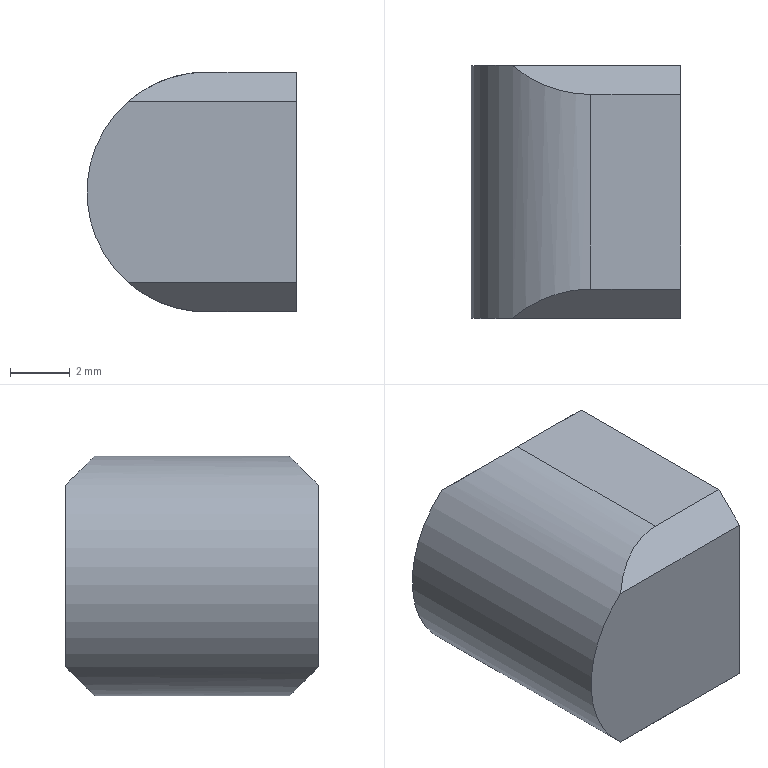Part | SolidWorks | features ICE 5, Chamfer 2, Extrusion 1, MoveFace 1 | 1 solid | 13 faces | box 7 x 8.44 x 8 mm | volume 333.679 mm3 | plane 10 | cylinder 3 | commonest cylinder face diameters 6.8 x2 8 x1
STEP:
#1=CARTESIAN_POINT('',(1.,0.,3.4));
#2=VERTEX_POINT('',#1);
#3=CARTESIAN_POINT('',(1.,0.,-3.4));
#4=VERTEX_POINT('',#3);
#5=CARTESIAN_POINT('',(1.,0.,0.));
#6=DIRECTION('',(1.,0.,0.));
#7=DIRECTION('',(0.,0.,-1.));
#8=AXIS2_PLACEMENT_3D('',#5,#6,#7);
#9=CIRCLE('',#8,3.4);
#10=EDGE_CURVE('',#2,#4,#9,.T.);
#11=ORIENTED_EDGE('',*,*,#10,.F.);
#12=CARTESIAN_POINT('',(3.,0.,3.4));
#13=VERTEX_POINT('',#12);
#14=CARTESIAN_POINT('',(1.,0.,3.4));
#15=DIRECTION('',(1.,0.,0.));
#16=VECTOR('',#15,1000.);
#17=LINE('',#14,#16);
#18=EDGE_CURVE('',#2,#13,#17,.T.);
#19=ORIENTED_EDGE('',*,*,#18,.T.);
#20=CARTESIAN_POINT('',(3.,0.,-3.4));
#21=VERTEX_POINT('',#20);
#22=CARTESIAN_POINT('',(3.,0.,0.));
#23=DIRECTION('',(1.,0.,0.));
#24=DIRECTION('',(0.,0.,-1.));
#25=AXIS2_PLACEMENT_3D('',#22,#23,#24);
#26=CIRCLE('',#25,3.4);
#27=EDGE_CURVE('',#13,#21,#26,.T.);
#28=ORIENTED_EDGE('',*,*,#27,.T.);
#29=CARTESIAN_POINT('',(1.,0.,-3.4));
#30=DIRECTION('',(1.,0.,0.));
#31=VECTOR('',#30,1000.);
#32=LINE('',#29,#31);
#33=EDGE_CURVE('',#4,#21,#32,.T.);
#34=ORIENTED_EDGE('',*,*,#33,.F.);
#35=EDGE_LOOP('',(#11,#19,#28,#34));
#36=FACE_OUTER_BOUND('',#35,.T.);
#37=CARTESIAN_POINT('',(1.,0.,0.));
#38=DIRECTION('',(1.,0.,0.));
#39=DIRECTION('',(0.,0.,-1.));
#40=AXIS2_PLACEMENT_3D('',#37,#38,#39);
#41=CYLINDRICAL_SURFACE('',#40,3.4);
#42=ADVANCED_FACE('',(#36),#41,.F.);
#43=CARTESIAN_POINT('',(-2.611,4.22,3.03));
#44=VERTEX_POINT('',#43);
#45=CARTESIAN_POINT('',(-2.611,4.22,-3.03));
#46=VERTEX_POINT('',#45);
#47=CARTESIAN_POINT('',(0.,4.22,0.));
#48=DIRECTION('',(0.,-1.,0.));
#49=DIRECTION('',(0.,0.,1.));
#50=AXIS2_PLACEMENT_3D('',#47,#48,#49);
#51=CIRCLE('',#50,4.);
#52=EDGE_CURVE('',#44,#46,#51,.T.);
#53=ORIENTED_EDGE('',*,*,#52,.F.);
#54=CARTESIAN_POINT('',(3.,4.22,3.03));
#55=VERTEX_POINT('',#54);
#56=CARTESIAN_POINT('',(0.,4.22,3.03));
#57=DIRECTION('',(1.,0.,0.));
#58=VECTOR('',#57,1000.);
#59=LINE('',#56,#58);
#60=EDGE_CURVE('',#44,#55,#59,.T.);
#61=ORIENTED_EDGE('',*,*,#60,.T.);
#62=CARTESIAN_POINT('',(3.,4.22,-3.03));
#63=VERTEX_POINT('',#62);
#64=CARTESIAN_POINT('',(3.,4.22,-4.));
#65=DIRECTION('',(0.,0.,-1.));
#66=VECTOR('',#65,1000.);
#67=LINE('',#64,#66);
#68=EDGE_CURVE('',#55,#63,#67,.T.);
#69=ORIENTED_EDGE('',*,*,#68,.T.);
#70=CARTESIAN_POINT('',(0.,4.22,-3.03));
#71=DIRECTION('',(-1.,0.,0.));
#72=VECTOR('',#71,1000.);
#73=LINE('',#70,#72);
#74=EDGE_CURVE('',#63,#46,#73,.T.);
#75=ORIENTED_EDGE('',*,*,#74,.T.);
#76=EDGE_LOOP('',(#53,#61,#69,#75));
#77=FACE_OUTER_BOUND('',#76,.T.);
#78=CARTESIAN_POINT('',(0.,4.22,0.));
#79=DIRECTION('',(0.,1.,0.));
#80=DIRECTION('',(0.,0.,1.));
#81=AXIS2_PLACEMENT_3D('',#78,#79,#80);
#82=PLANE('',#81);
#83=ADVANCED_FACE('',(#77),#82,.T.);
#84=CARTESIAN_POINT('',(3.,-4.22,3.03));
#85=VERTEX_POINT('',#84);
#86=CARTESIAN_POINT('',(-2.611,-4.22,3.03));
#87=VERTEX_POINT('',#86);
#88=CARTESIAN_POINT('',(0.,-4.22,3.03));
#89=DIRECTION('',(-1.,0.,0.));
#90=VECTOR('',#89,1000.);
#91=LINE('',#88,#90);
#92=EDGE_CURVE('',#85,#87,#91,.T.);
#93=ORIENTED_EDGE('',*,*,#92,.T.);
#94=CARTESIAN_POINT('',(-2.611,-4.22,-3.03));
#95=VERTEX_POINT('',#94);
#96=CARTESIAN_POINT('',(0.,-4.22,0.));
#97=DIRECTION('',(0.,1.,0.));
#98=DIRECTION('',(0.,0.,1.));
#99=AXIS2_PLACEMENT_3D('',#96,#97,#98);
#100=CIRCLE('',#99,4.);
#101=EDGE_CURVE('',#95,#87,#100,.T.);
#102=ORIENTED_EDGE('',*,*,#101,.F.);
#103=CARTESIAN_POINT('',(3.,-4.22,-3.03));
#104=VERTEX_POINT('',#103);
#105=CARTESIAN_POINT('',(0.,-4.22,-3.03));
#106=DIRECTION('',(1.,0.,0.));
#107=VECTOR('',#106,1000.);
#108=LINE('',#105,#107);
#109=EDGE_CURVE('',#95,#104,#108,.T.);
#110=ORIENTED_EDGE('',*,*,#109,.T.);
#111=CARTESIAN_POINT('',(3.,-4.22,-4.));
#112=DIRECTION('',(0.,0.,-1.));
#113=VECTOR('',#112,1000.);
#114=LINE('',#111,#113);
#115=EDGE_CURVE('',#85,#104,#114,.T.);
#116=ORIENTED_EDGE('',*,*,#115,.F.);
#117=EDGE_LOOP('',(#93,#102,#110,#116));
#118=FACE_OUTER_BOUND('',#117,.T.);
#119=CARTESIAN_POINT('',(0.,-4.22,0.));
#120=DIRECTION('',(0.,1.,0.));
#121=DIRECTION('',(0.,0.,1.));
#122=AXIS2_PLACEMENT_3D('',#119,#120,#121);
#123=PLANE('',#122);
#124=ADVANCED_FACE('',(#118),#123,.F.);
#125=CARTESIAN_POINT('',(0.,3.25,-4.));
#126=VERTEX_POINT('',#125);
#127=CARTESIAN_POINT('',(-2.611,4.22,-3.03));
#128=CARTESIAN_POINT('',(-1.877,3.587,-3.663));
#129=CARTESIAN_POINT('',(-0.969,3.25,-4.));
#130=CARTESIAN_POINT('',(0.,3.25,-4.));
#131=(BOUNDED_CURVE()B_SPLINE_CURVE(3,(#127,#128,#129,#130),.UNSPECIFIED.,.F.,.F.)B_SPLINE_CURVE_WITH_KNOTS((4,4),(5.572,6.283),.UNSPECIFIED.)CURVE()GEOMETRIC_REPRESENTATION_ITEM()RATIONAL_B_SPLINE_CURVE((1.,0.9583,0.9583,1.))REPRESENTATION_ITEM(''));
#132=EDGE_CURVE('',#46,#126,#131,.T.);
#133=ORIENTED_EDGE('',*,*,#132,.F.);
#134=ORIENTED_EDGE('',*,*,#74,.F.);
#135=CARTESIAN_POINT('',(3.,3.25,-4.));
#136=VERTEX_POINT('',#135);
#137=CARTESIAN_POINT('',(3.,4.25,-3.));
#138=DIRECTION('',(0.,0.7071,0.7071));
#139=VECTOR('',#138,1000.);
#140=LINE('',#137,#139);
#141=EDGE_CURVE('',#136,#63,#140,.T.);
#142=ORIENTED_EDGE('',*,*,#141,.F.);
#143=CARTESIAN_POINT('',(3.,3.25,-4.));
#144=DIRECTION('',(1.,0.,0.));
#145=VECTOR('',#144,1000.);
#146=LINE('',#143,#145);
#147=EDGE_CURVE('',#126,#136,#146,.T.);
#148=ORIENTED_EDGE('',*,*,#147,.F.);
#149=EDGE_LOOP('',(#133,#134,#142,#148));
#150=FACE_OUTER_BOUND('',#149,.T.);
#151=CARTESIAN_POINT('',(0.,4.25,-3.));
#152=DIRECTION('',(0.,0.7071,-0.7071));
#153=DIRECTION('',(1.,0.,0.));
#154=AXIS2_PLACEMENT_3D('',#151,#152,#153);
#155=PLANE('',#154);
#156=ADVANCED_FACE('',(#150),#155,.T.);
#157=CARTESIAN_POINT('',(0.,3.25,4.));
#158=VERTEX_POINT('',#157);
#159=CARTESIAN_POINT('',(0.,3.25,4.));
#160=CARTESIAN_POINT('',(-0.969,3.25,4.));
#161=CARTESIAN_POINT('',(-1.877,3.587,3.663));
#162=CARTESIAN_POINT('',(-2.611,4.22,3.03));
#163=(BOUNDED_CURVE()B_SPLINE_CURVE(3,(#159,#160,#161,#162),.UNSPECIFIED.,.F.,.T.)B_SPLINE_CURVE_WITH_KNOTS((4,4),(0.,0.7113),.UNSPECIFIED.)CURVE()GEOMETRIC_REPRESENTATION_ITEM()RATIONAL_B_SPLINE_CURVE((1.,0.9583,0.9583,1.))REPRESENTATION_ITEM(''));
#164=EDGE_CURVE('',#158,#44,#163,.T.);
#165=ORIENTED_EDGE('',*,*,#164,.F.);
#166=CARTESIAN_POINT('',(3.,3.25,4.));
#167=VERTEX_POINT('',#166);
#168=CARTESIAN_POINT('',(-4.,3.25,4.));
#169=DIRECTION('',(-1.,0.,0.));
#170=VECTOR('',#169,1000.);
#171=LINE('',#168,#170);
#172=EDGE_CURVE('',#167,#158,#171,.T.);
#173=ORIENTED_EDGE('',*,*,#172,.F.);
#174=CARTESIAN_POINT('',(3.,4.25,3.));
#175=DIRECTION('',(0.,-0.7071,0.7071));
#176=VECTOR('',#175,1000.);
#177=LINE('',#174,#176);
#178=EDGE_CURVE('',#55,#167,#177,.T.);
#179=ORIENTED_EDGE('',*,*,#178,.F.);
#180=ORIENTED_EDGE('',*,*,#60,.F.);
#181=EDGE_LOOP('',(#165,#173,#179,#180));
#182=FACE_OUTER_BOUND('',#181,.T.);
#183=CARTESIAN_POINT('',(0.,4.25,3.));
#184=DIRECTION('',(0.,0.7071,0.7071));
#185=DIRECTION('',(-1.,0.,0.));
#186=AXIS2_PLACEMENT_3D('',#183,#184,#185);
#187=PLANE('',#186);
#188=ADVANCED_FACE('',(#182),#187,.T.);
#189=ORIENTED_EDGE('',*,*,#172,.T.);
#190=CARTESIAN_POINT('',(0.,-3.25,4.));
#191=VERTEX_POINT('',#190);
#192=CARTESIAN_POINT('',(0.,53.75,4.));
#193=DIRECTION('',(0.,-1.,0.));
#194=VECTOR('',#193,1000.);
#195=LINE('',#192,#194);
#196=EDGE_CURVE('',#158,#191,#195,.T.);
#197=ORIENTED_EDGE('',*,*,#196,.T.);
#198=CARTESIAN_POINT('',(3.,-3.25,4.));
#199=VERTEX_POINT('',#198);
#200=CARTESIAN_POINT('',(0.,-3.25,4.));
#201=DIRECTION('',(1.,0.,0.));
#202=VECTOR('',#201,1000.);
#203=LINE('',#200,#202);
#204=EDGE_CURVE('',#191,#199,#203,.T.);
#205=ORIENTED_EDGE('',*,*,#204,.T.);
#206=CARTESIAN_POINT('',(3.,4.25,4.));
#207=DIRECTION('',(0.,-1.,0.));
#208=VECTOR('',#207,1000.);
#209=LINE('',#206,#208);
#210=EDGE_CURVE('',#167,#199,#209,.T.);
#211=ORIENTED_EDGE('',*,*,#210,.F.);
#212=EDGE_LOOP('',(#189,#197,#205,#211));
#213=FACE_OUTER_BOUND('',#212,.T.);
#214=CARTESIAN_POINT('',(0.,4.25,4.));
#215=DIRECTION('',(0.,0.,-1.));
#216=DIRECTION('',(-1.,0.,0.));
#217=AXIS2_PLACEMENT_3D('',#214,#215,#216);
#218=PLANE('',#217);
#219=ADVANCED_FACE('',(#213),#218,.F.);
#220=CARTESIAN_POINT('',(3.,0.,0.));
#221=DIRECTION('',(1.,0.,0.));
#222=DIRECTION('',(0.,0.,-1.));
#223=AXIS2_PLACEMENT_3D('',#220,#221,#222);
#224=CIRCLE('',#223,3.4);
#225=EDGE_CURVE('',#21,#13,#224,.T.);
#226=ORIENTED_EDGE('',*,*,#225,.F.);
#227=ORIENTED_EDGE('',*,*,#27,.F.);
#228=EDGE_LOOP('',(#226,#227));
#229=FACE_BOUND('',#228,.T.);
#230=CARTESIAN_POINT('',(3.,-3.25,-4.));
#231=VERTEX_POINT('',#230);
#232=CARTESIAN_POINT('',(3.,4.25,-4.));
#233=DIRECTION('',(0.,-1.,0.));
#234=VECTOR('',#233,1000.);
#235=LINE('',#232,#234);
#236=EDGE_CURVE('',#136,#231,#235,.T.);
#237=ORIENTED_EDGE('',*,*,#236,.F.);
#238=ORIENTED_EDGE('',*,*,#141,.T.);
#239=ORIENTED_EDGE('',*,*,#68,.F.);
#240=ORIENTED_EDGE('',*,*,#178,.T.);
#241=ORIENTED_EDGE('',*,*,#210,.T.);
#242=CARTESIAN_POINT('',(3.,-3.25,4.));
#243=DIRECTION('',(0.,-0.7071,-0.7071));
#244=VECTOR('',#243,1000.);
#245=LINE('',#242,#244);
#246=EDGE_CURVE('',#199,#85,#245,.T.);
#247=ORIENTED_EDGE('',*,*,#246,.T.);
#248=ORIENTED_EDGE('',*,*,#115,.T.);
#249=CARTESIAN_POINT('',(3.,-3.25,-4.));
#250=DIRECTION('',(0.,0.7071,-0.7071));
#251=VECTOR('',#250,1000.);
#252=LINE('',#249,#251);
#253=EDGE_CURVE('',#104,#231,#252,.T.);
#254=ORIENTED_EDGE('',*,*,#253,.T.);
#255=EDGE_LOOP('',(#237,#238,#239,#240,#241,#247,#248,#254));
#256=FACE_OUTER_BOUND('',#255,.T.);
#257=CARTESIAN_POINT('',(3.,4.25,-4.));
#258=DIRECTION('',(-1.,0.,0.));
#259=DIRECTION('',(0.,0.,1.));
#260=AXIS2_PLACEMENT_3D('',#257,#258,#259);
#261=PLANE('',#260);
#262=ADVANCED_FACE('',(#229,#256),#261,.F.);
#263=CARTESIAN_POINT('',(0.,-3.25,-4.));
#264=VERTEX_POINT('',#263);
#265=CARTESIAN_POINT('',(0.,-3.25,-4.));
#266=DIRECTION('',(-1.,0.,0.));
#267=VECTOR('',#266,1000.);
#268=LINE('',#265,#267);
#269=EDGE_CURVE('',#231,#264,#268,.T.);
#270=ORIENTED_EDGE('',*,*,#269,.T.);
#271=CARTESIAN_POINT('',(0.,53.75,-4.));
#272=DIRECTION('',(0.,-1.,0.));
#273=VECTOR('',#272,1000.);
#274=LINE('',#271,#273);
#275=EDGE_CURVE('',#126,#264,#274,.T.);
#276=ORIENTED_EDGE('',*,*,#275,.F.);
#277=ORIENTED_EDGE('',*,*,#147,.T.);
#278=ORIENTED_EDGE('',*,*,#236,.T.);
#279=EDGE_LOOP('',(#270,#276,#277,#278));
#280=FACE_OUTER_BOUND('',#279,.T.);
#281=CARTESIAN_POINT('',(0.,4.25,-4.));
#282=DIRECTION('',(0.,0.,1.));
#283=DIRECTION('',(1.,0.,0.));
#284=AXIS2_PLACEMENT_3D('',#281,#282,#283);
#285=PLANE('',#284);
#286=ADVANCED_FACE('',(#280),#285,.F.);
#287=ORIENTED_EDGE('',*,*,#18,.F.);
#288=CARTESIAN_POINT('',(1.,0.,0.));
#289=DIRECTION('',(1.,0.,0.));
#290=DIRECTION('',(0.,0.,-1.));
#291=AXIS2_PLACEMENT_3D('',#288,#289,#290);
#292=CIRCLE('',#291,3.4);
#293=EDGE_CURVE('',#4,#2,#292,.T.);
#294=ORIENTED_EDGE('',*,*,#293,.F.);
#295=ORIENTED_EDGE('',*,*,#33,.T.);
#296=ORIENTED_EDGE('',*,*,#225,.T.);
#297=EDGE_LOOP('',(#287,#294,#295,#296));
#298=FACE_OUTER_BOUND('',#297,.T.);
#299=CARTESIAN_POINT('',(1.,0.,0.));
#300=DIRECTION('',(1.,0.,0.));
#301=DIRECTION('',(0.,0.,-1.));
#302=AXIS2_PLACEMENT_3D('',#299,#300,#301);
#303=CYLINDRICAL_SURFACE('',#302,3.4);
#304=ADVANCED_FACE('',(#298),#303,.F.);
#305=ORIENTED_EDGE('',*,*,#293,.T.);
#306=ORIENTED_EDGE('',*,*,#10,.T.);
#307=EDGE_LOOP('',(#305,#306));
#308=FACE_OUTER_BOUND('',#307,.T.);
#309=CARTESIAN_POINT('',(1.,0.,0.));
#310=DIRECTION('',(1.,0.,0.));
#311=DIRECTION('',(0.,0.,-1.));
#312=AXIS2_PLACEMENT_3D('',#309,#310,#311);
#313=PLANE('',#312);
#314=ADVANCED_FACE('',(#308),#313,.T.);
#315=CARTESIAN_POINT('',(0.,-3.25,-4.));
#316=CARTESIAN_POINT('',(-0.969,-3.25,-4.));
#317=CARTESIAN_POINT('',(-1.877,-3.587,-3.663));
#318=CARTESIAN_POINT('',(-2.611,-4.22,-3.03));
#319=(BOUNDED_CURVE()B_SPLINE_CURVE(3,(#315,#316,#317,#318),.UNSPECIFIED.,.F.,.F.)B_SPLINE_CURVE_WITH_KNOTS((4,4),(3.142,3.853),.UNSPECIFIED.)CURVE()GEOMETRIC_REPRESENTATION_ITEM()RATIONAL_B_SPLINE_CURVE((1.,0.9583,0.9583,1.))REPRESENTATION_ITEM(''));
#320=EDGE_CURVE('',#264,#95,#319,.T.);
#321=ORIENTED_EDGE('',*,*,#320,.F.);
#322=ORIENTED_EDGE('',*,*,#269,.F.);
#323=ORIENTED_EDGE('',*,*,#253,.F.);
#324=ORIENTED_EDGE('',*,*,#109,.F.);
#325=EDGE_LOOP('',(#321,#322,#323,#324));
#326=FACE_OUTER_BOUND('',#325,.T.);
#327=CARTESIAN_POINT('',(0.,-3.25,-4.));
#328=DIRECTION('',(0.,0.7071,0.7071));
#329=DIRECTION('',(-1.,0.,0.));
#330=AXIS2_PLACEMENT_3D('',#327,#328,#329);
#331=PLANE('',#330);
#332=ADVANCED_FACE('',(#326),#331,.F.);
#333=CARTESIAN_POINT('',(-2.611,-4.22,3.03));
#334=CARTESIAN_POINT('',(-1.877,-3.587,3.663));
#335=CARTESIAN_POINT('',(-0.969,-3.25,4.));
#336=CARTESIAN_POINT('',(0.,-3.25,4.));
#337=(BOUNDED_CURVE()B_SPLINE_CURVE(3,(#333,#334,#335,#336),.UNSPECIFIED.,.F.,.T.)B_SPLINE_CURVE_WITH_KNOTS((4,4),(2.43,3.142),.UNSPECIFIED.)CURVE()GEOMETRIC_REPRESENTATION_ITEM()RATIONAL_B_SPLINE_CURVE((1.,0.9583,0.9583,1.))REPRESENTATION_ITEM(''));
#338=EDGE_CURVE('',#87,#191,#337,.T.);
#339=ORIENTED_EDGE('',*,*,#338,.F.);
#340=ORIENTED_EDGE('',*,*,#92,.F.);
#341=ORIENTED_EDGE('',*,*,#246,.F.);
#342=ORIENTED_EDGE('',*,*,#204,.F.);
#343=EDGE_LOOP('',(#339,#340,#341,#342));
#344=FACE_OUTER_BOUND('',#343,.T.);
#345=CARTESIAN_POINT('',(0.,-3.25,4.));
#346=DIRECTION('',(0.,0.7071,-0.7071));
#347=DIRECTION('',(1.,0.,0.));
#348=AXIS2_PLACEMENT_3D('',#345,#346,#347);
#349=PLANE('',#348);
#350=ADVANCED_FACE('',(#344),#349,.F.);
#351=ORIENTED_EDGE('',*,*,#101,.T.);
#352=ORIENTED_EDGE('',*,*,#338,.T.);
#353=ORIENTED_EDGE('',*,*,#196,.F.);
#354=ORIENTED_EDGE('',*,*,#164,.T.);
#355=ORIENTED_EDGE('',*,*,#52,.T.);
#356=ORIENTED_EDGE('',*,*,#132,.T.);
#357=ORIENTED_EDGE('',*,*,#275,.T.);
#358=ORIENTED_EDGE('',*,*,#320,.T.);
#359=EDGE_LOOP('',(#351,#352,#353,#354,#355,#356,#357,#358));
#360=FACE_OUTER_BOUND('',#359,.T.);
#361=CARTESIAN_POINT('',(0.,53.75,0.));
#362=DIRECTION('',(0.,-1.,0.));
#363=DIRECTION('',(0.,0.,-1.));
#364=AXIS2_PLACEMENT_3D('',#361,#362,#363);
#365=CYLINDRICAL_SURFACE('',#364,4.);
#366=ADVANCED_FACE('',(#360),#365,.T.);
#367=CLOSED_SHELL('',(#42,#83,#124,#156,#188,#219,#262,#286,#304,#314,#332,#350,#366));
#368=MANIFOLD_SOLID_BREP('',#367);
#369=CARTESIAN_POINT('',(0.,0.,0.));
#370=DIRECTION('',(0.,0.,1.));
#371=DIRECTION('',(1.,0.,0.));
#372=AXIS2_PLACEMENT_3D('',#369,#370,#371);
#373=(LENGTH_UNIT()NAMED_UNIT(*)SI_UNIT(.MILLI.,.METRE.));
#374=UNCERTAINTY_MEASURE_WITH_UNIT(LENGTH_MEASURE(0.00001),#373,'','');
#375=(NAMED_UNIT(*)PLANE_ANGLE_UNIT()SI_UNIT($,.RADIAN.));
#376=(NAMED_UNIT(*)SI_UNIT($,.STERADIAN.)SOLID_ANGLE_UNIT());
#377=(GEOMETRIC_REPRESENTATION_CONTEXT(3)GLOBAL_UNCERTAINTY_ASSIGNED_CONTEXT((#374))GLOBAL_UNIT_ASSIGNED_CONTEXT((#373,#375,#376))REPRESENTATION_CONTEXT('',''));
#378=ADVANCED_BREP_SHAPE_REPRESENTATION('',(#368,#372),#377);